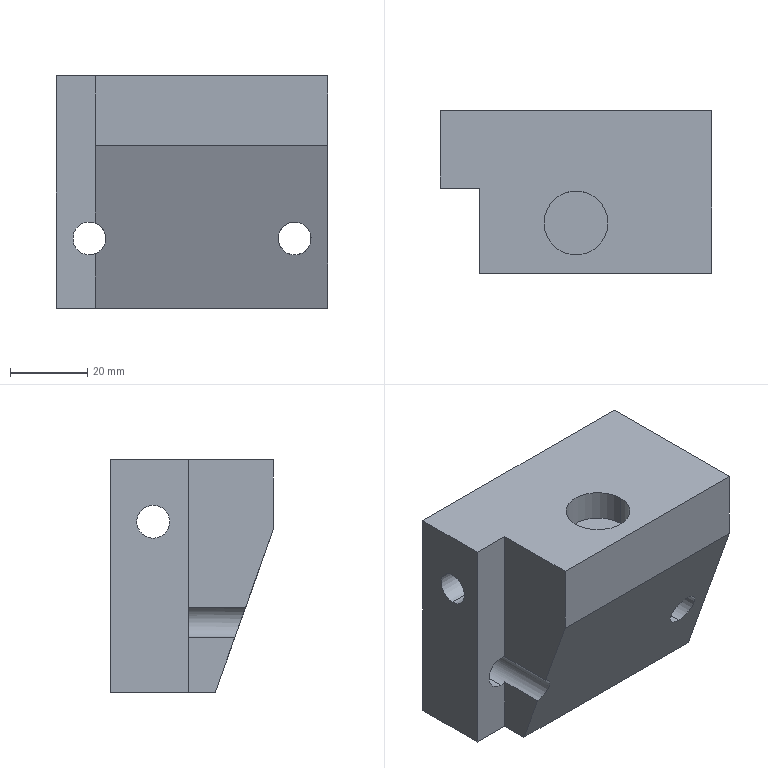Part | SolidWorks | features ICE 4, Extrusion 1 | 1 solid | 19 faces | box 70 x 42 x 60 mm | volume 135372 mm3 | plane 11 | cylinder 8 | commonest cylinder face diameters 8.5 x6 16.5 x2
STEP:
#1=CARTESIAN_POINT('',(-8.25,-9.,22.));
#2=VERTEX_POINT('',#1);
#3=CARTESIAN_POINT('',(8.25,-9.,22.));
#4=VERTEX_POINT('',#3);
#5=CARTESIAN_POINT('',(0.,-9.,22.));
#6=DIRECTION('',(0.,0.,1.));
#7=DIRECTION('',(1.,0.,0.));
#8=AXIS2_PLACEMENT_3D('',#5,#6,#7);
#9=CIRCLE('',#8,8.25);
#10=EDGE_CURVE('',#2,#4,#9,.T.);
#11=ORIENTED_EDGE('',*,*,#10,.F.);
#12=CARTESIAN_POINT('',(-8.25,-9.,30.));
#13=VERTEX_POINT('',#12);
#14=CARTESIAN_POINT('',(-8.25,-9.,22.));
#15=DIRECTION('',(0.,0.,1.));
#16=VECTOR('',#15,1000.);
#17=LINE('',#14,#16);
#18=EDGE_CURVE('',#2,#13,#17,.T.);
#19=ORIENTED_EDGE('',*,*,#18,.T.);
#20=CARTESIAN_POINT('',(8.25,-9.,30.));
#21=VERTEX_POINT('',#20);
#22=CARTESIAN_POINT('',(0.,-9.,30.));
#23=DIRECTION('',(0.,0.,1.));
#24=DIRECTION('',(1.,0.,0.));
#25=AXIS2_PLACEMENT_3D('',#22,#23,#24);
#26=CIRCLE('',#25,8.25);
#27=EDGE_CURVE('',#13,#21,#26,.T.);
#28=ORIENTED_EDGE('',*,*,#27,.T.);
#29=CARTESIAN_POINT('',(8.25,-9.,22.));
#30=DIRECTION('',(0.,0.,1.));
#31=VECTOR('',#30,1000.);
#32=LINE('',#29,#31);
#33=EDGE_CURVE('',#4,#21,#32,.T.);
#34=ORIENTED_EDGE('',*,*,#33,.F.);
#35=EDGE_LOOP('',(#11,#19,#28,#34));
#36=FACE_OUTER_BOUND('',#35,.T.);
#37=CARTESIAN_POINT('',(0.,-9.,22.));
#38=DIRECTION('',(0.,0.,1.));
#39=DIRECTION('',(1.,0.,0.));
#40=AXIS2_PLACEMENT_3D('',#37,#38,#39);
#41=CYLINDRICAL_SURFACE('',#40,8.25);
#42=ADVANCED_FACE('',(#36),#41,.F.);
#43=CARTESIAN_POINT('',(26.5,-14.946,-7.75));
#44=VERTEX_POINT('',#43);
#45=CARTESIAN_POINT('',(26.5,-11.911,-16.25));
#46=VERTEX_POINT('',#45);
#47=CARTESIAN_POINT('',(26.5,-14.946,-7.75));
#48=CARTESIAN_POINT('',(18.,-14.946,-7.75));
#49=CARTESIAN_POINT('',(18.,-11.911,-16.25));
#50=CARTESIAN_POINT('',(26.5,-11.911,-16.25));
#51=(BOUNDED_CURVE()B_SPLINE_CURVE(3,(#47,#48,#49,#50),.UNSPECIFIED.,.F.,.F.)B_SPLINE_CURVE_WITH_KNOTS((4,4),(3.142,6.283),.UNSPECIFIED.)CURVE()GEOMETRIC_REPRESENTATION_ITEM()RATIONAL_B_SPLINE_CURVE((1.,0.3333,0.3333,1.))REPRESENTATION_ITEM(''));
#52=EDGE_CURVE('',#44,#46,#51,.T.);
#53=ORIENTED_EDGE('',*,*,#52,.T.);
#54=CARTESIAN_POINT('',(26.5,20.,-16.25));
#55=VERTEX_POINT('',#54);
#56=CARTESIAN_POINT('',(26.5,-71.,-16.25));
#57=DIRECTION('',(0.,1.,0.));
#58=VECTOR('',#57,1000.);
#59=LINE('',#56,#58);
#60=EDGE_CURVE('',#46,#55,#59,.T.);
#61=ORIENTED_EDGE('',*,*,#60,.T.);
#62=CARTESIAN_POINT('',(26.5,20.,-7.75));
#63=VERTEX_POINT('',#62);
#64=CARTESIAN_POINT('',(26.5,20.,-12.));
#65=DIRECTION('',(0.,1.,0.));
#66=DIRECTION('',(0.,0.,1.));
#67=AXIS2_PLACEMENT_3D('',#64,#65,#66);
#68=CIRCLE('',#67,4.25);
#69=EDGE_CURVE('',#55,#63,#68,.T.);
#70=ORIENTED_EDGE('',*,*,#69,.T.);
#71=CARTESIAN_POINT('',(26.5,-71.,-7.75));
#72=DIRECTION('',(0.,1.,0.));
#73=VECTOR('',#72,1000.);
#74=LINE('',#71,#73);
#75=EDGE_CURVE('',#44,#63,#74,.T.);
#76=ORIENTED_EDGE('',*,*,#75,.F.);
#77=EDGE_LOOP('',(#53,#61,#70,#76));
#78=FACE_OUTER_BOUND('',#77,.T.);
#79=CARTESIAN_POINT('',(26.5,-71.,-12.));
#80=DIRECTION('',(0.,1.,0.));
#81=DIRECTION('',(0.,0.,1.));
#82=AXIS2_PLACEMENT_3D('',#79,#80,#81);
#83=CYLINDRICAL_SURFACE('',#82,4.25);
#84=ADVANCED_FACE('',(#78),#83,.F.);
#85=CARTESIAN_POINT('',(-26.5,0.,-16.25));
#86=VERTEX_POINT('',#85);
#87=CARTESIAN_POINT('',(-26.5,0.,-7.75));
#88=VERTEX_POINT('',#87);
#89=CARTESIAN_POINT('',(-26.5,0.,-12.));
#90=DIRECTION('',(0.,1.,0.));
#91=DIRECTION('',(0.,0.,1.));
#92=AXIS2_PLACEMENT_3D('',#89,#90,#91);
#93=CIRCLE('',#92,4.25);
#94=EDGE_CURVE('',#86,#88,#93,.T.);
#95=ORIENTED_EDGE('',*,*,#94,.F.);
#96=CARTESIAN_POINT('',(-26.5,20.,-16.25));
#97=VERTEX_POINT('',#96);
#98=CARTESIAN_POINT('',(-26.5,-71.,-16.25));
#99=DIRECTION('',(0.,1.,0.));
#100=VECTOR('',#99,1000.);
#101=LINE('',#98,#100);
#102=EDGE_CURVE('',#86,#97,#101,.T.);
#103=ORIENTED_EDGE('',*,*,#102,.T.);
#104=CARTESIAN_POINT('',(-26.5,20.,-7.75));
#105=VERTEX_POINT('',#104);
#106=CARTESIAN_POINT('',(-26.5,20.,-12.));
#107=DIRECTION('',(0.,1.,0.));
#108=DIRECTION('',(0.,0.,-1.));
#109=AXIS2_PLACEMENT_3D('',#106,#107,#108);
#110=CIRCLE('',#109,4.25);
#111=EDGE_CURVE('',#97,#105,#110,.T.);
#112=ORIENTED_EDGE('',*,*,#111,.T.);
#113=CARTESIAN_POINT('',(-26.5,-71.,-7.75));
#114=DIRECTION('',(0.,1.,0.));
#115=VECTOR('',#114,1000.);
#116=LINE('',#113,#115);
#117=EDGE_CURVE('',#88,#105,#116,.T.);
#118=ORIENTED_EDGE('',*,*,#117,.F.);
#119=EDGE_LOOP('',(#95,#103,#112,#118));
#120=FACE_OUTER_BOUND('',#119,.T.);
#121=CARTESIAN_POINT('',(-26.5,-71.,-12.));
#122=DIRECTION('',(0.,1.,0.));
#123=DIRECTION('',(0.,0.,1.));
#124=AXIS2_PLACEMENT_3D('',#121,#122,#123);
#125=CYLINDRICAL_SURFACE('',#124,4.25);
#126=ADVANCED_FACE('',(#120),#125,.F.);
#127=CARTESIAN_POINT('',(35.,9.,9.75));
#128=VERTEX_POINT('',#127);
#129=CARTESIAN_POINT('',(35.,9.,18.25));
#130=VERTEX_POINT('',#129);
#131=CARTESIAN_POINT('',(35.,9.,14.));
#132=DIRECTION('',(-1.,0.,0.));
#133=DIRECTION('',(0.,0.,1.));
#134=AXIS2_PLACEMENT_3D('',#131,#132,#133);
#135=CIRCLE('',#134,4.25);
#136=EDGE_CURVE('',#128,#130,#135,.T.);
#137=ORIENTED_EDGE('',*,*,#136,.F.);
#138=CARTESIAN_POINT('',(-35.,9.,9.75));
#139=VERTEX_POINT('',#138);
#140=CARTESIAN_POINT('',(96.,9.,9.75));
#141=DIRECTION('',(-1.,0.,0.));
#142=VECTOR('',#141,1000.);
#143=LINE('',#140,#142);
#144=EDGE_CURVE('',#128,#139,#143,.T.);
#145=ORIENTED_EDGE('',*,*,#144,.T.);
#146=CARTESIAN_POINT('',(-35.,9.,18.25));
#147=VERTEX_POINT('',#146);
#148=CARTESIAN_POINT('',(-35.,9.,14.));
#149=DIRECTION('',(-1.,0.,0.));
#150=DIRECTION('',(0.,0.,1.));
#151=AXIS2_PLACEMENT_3D('',#148,#149,#150);
#152=CIRCLE('',#151,4.25);
#153=EDGE_CURVE('',#139,#147,#152,.T.);
#154=ORIENTED_EDGE('',*,*,#153,.T.);
#155=CARTESIAN_POINT('',(96.,9.,18.25));
#156=DIRECTION('',(-1.,0.,0.));
#157=VECTOR('',#156,1000.);
#158=LINE('',#155,#157);
#159=EDGE_CURVE('',#130,#147,#158,.T.);
#160=ORIENTED_EDGE('',*,*,#159,.F.);
#161=EDGE_LOOP('',(#137,#145,#154,#160));
#162=FACE_OUTER_BOUND('',#161,.T.);
#163=CARTESIAN_POINT('',(96.,9.,14.));
#164=DIRECTION('',(-1.,0.,0.));
#165=DIRECTION('',(0.,0.,1.));
#166=AXIS2_PLACEMENT_3D('',#163,#164,#165);
#167=CYLINDRICAL_SURFACE('',#166,4.25);
#168=ADVANCED_FACE('',(#162),#167,.F.);
#169=CARTESIAN_POINT('',(-25.,-14.849,-8.024));
#170=VERTEX_POINT('',#169);
#171=CARTESIAN_POINT('',(-25.,0.,-8.024));
#172=VERTEX_POINT('',#171);
#173=CARTESIAN_POINT('',(-25.,-71.,-8.024));
#174=DIRECTION('',(0.,1.,0.));
#175=VECTOR('',#174,1000.);
#176=LINE('',#173,#175);
#177=EDGE_CURVE('',#170,#172,#176,.T.);
#178=ORIENTED_EDGE('',*,*,#177,.F.);
#179=CARTESIAN_POINT('',(-25.,-22.,12.));
#180=VERTEX_POINT('',#179);
#181=CARTESIAN_POINT('',(-25.,-7.,-30.));
#182=DIRECTION('',(0.,0.3363,-0.9417));
#183=VECTOR('',#182,1000.);
#184=LINE('',#181,#183);
#185=EDGE_CURVE('',#180,#170,#184,.T.);
#186=ORIENTED_EDGE('',*,*,#185,.F.);
#187=CARTESIAN_POINT('',(-25.,-22.,30.));
#188=VERTEX_POINT('',#187);
#189=CARTESIAN_POINT('',(-25.,-22.,12.));
#190=DIRECTION('',(0.,0.,-1.));
#191=VECTOR('',#190,1000.);
#192=LINE('',#189,#191);
#193=EDGE_CURVE('',#188,#180,#192,.T.);
#194=ORIENTED_EDGE('',*,*,#193,.F.);
#195=CARTESIAN_POINT('',(-25.,0.,30.));
#196=VERTEX_POINT('',#195);
#197=CARTESIAN_POINT('',(-25.,-22.,30.));
#198=DIRECTION('',(0.,-1.,0.));
#199=VECTOR('',#198,1000.);
#200=LINE('',#197,#199);
#201=EDGE_CURVE('',#196,#188,#200,.T.);
#202=ORIENTED_EDGE('',*,*,#201,.F.);
#203=CARTESIAN_POINT('',(-25.,0.,0.));
#204=DIRECTION('',(0.,0.,1.));
#205=VECTOR('',#204,1000.);
#206=LINE('',#203,#205);
#207=EDGE_CURVE('',#172,#196,#206,.T.);
#208=ORIENTED_EDGE('',*,*,#207,.F.);
#209=EDGE_LOOP('',(#178,#186,#194,#202,#208));
#210=FACE_OUTER_BOUND('',#209,.T.);
#211=CARTESIAN_POINT('',(-25.,0.,0.));
#212=DIRECTION('',(-1.,0.,0.));
#213=DIRECTION('',(0.,0.,1.));
#214=AXIS2_PLACEMENT_3D('',#211,#212,#213);
#215=PLANE('',#214);
#216=ADVANCED_FACE('',(#210),#215,.T.);
#217=CARTESIAN_POINT('',(35.,9.,14.));
#218=DIRECTION('',(-1.,0.,0.));
#219=DIRECTION('',(0.,0.,1.));
#220=AXIS2_PLACEMENT_3D('',#217,#218,#219);
#221=CIRCLE('',#220,4.25);
#222=EDGE_CURVE('',#130,#128,#221,.T.);
#223=ORIENTED_EDGE('',*,*,#222,.T.);
#224=ORIENTED_EDGE('',*,*,#136,.T.);
#225=EDGE_LOOP('',(#223,#224));
#226=FACE_BOUND('',#225,.T.);
#227=CARTESIAN_POINT('',(35.,20.,30.));
#228=VERTEX_POINT('',#227);
#229=CARTESIAN_POINT('',(35.,-22.,30.));
#230=VERTEX_POINT('',#229);
#231=CARTESIAN_POINT('',(35.,20.,30.));
#232=DIRECTION('',(0.,-1.,0.));
#233=VECTOR('',#232,1000.);
#234=LINE('',#231,#233);
#235=EDGE_CURVE('',#228,#230,#234,.T.);
#236=ORIENTED_EDGE('',*,*,#235,.T.);
#237=CARTESIAN_POINT('',(35.,-22.,12.));
#238=VERTEX_POINT('',#237);
#239=CARTESIAN_POINT('',(35.,-22.,12.));
#240=DIRECTION('',(0.,0.,-1.));
#241=VECTOR('',#240,1000.);
#242=LINE('',#239,#241);
#243=EDGE_CURVE('',#230,#238,#242,.T.);
#244=ORIENTED_EDGE('',*,*,#243,.T.);
#245=CARTESIAN_POINT('',(35.,-7.,-30.));
#246=VERTEX_POINT('',#245);
#247=CARTESIAN_POINT('',(35.,-7.,-30.));
#248=DIRECTION('',(0.,0.3363,-0.9417));
#249=VECTOR('',#248,1000.);
#250=LINE('',#247,#249);
#251=EDGE_CURVE('',#238,#246,#250,.T.);
#252=ORIENTED_EDGE('',*,*,#251,.T.);
#253=CARTESIAN_POINT('',(35.,20.,-30.));
#254=VERTEX_POINT('',#253);
#255=CARTESIAN_POINT('',(35.,20.,-30.));
#256=DIRECTION('',(0.,-1.,0.));
#257=VECTOR('',#256,1000.);
#258=LINE('',#255,#257);
#259=EDGE_CURVE('',#254,#246,#258,.T.);
#260=ORIENTED_EDGE('',*,*,#259,.F.);
#261=CARTESIAN_POINT('',(35.,20.,-30.));
#262=DIRECTION('',(0.,0.,-1.));
#263=VECTOR('',#262,1000.);
#264=LINE('',#261,#263);
#265=EDGE_CURVE('',#228,#254,#264,.T.);
#266=ORIENTED_EDGE('',*,*,#265,.F.);
#267=EDGE_LOOP('',(#236,#244,#252,#260,#266));
#268=FACE_OUTER_BOUND('',#267,.T.);
#269=CARTESIAN_POINT('',(35.,20.,-30.));
#270=DIRECTION('',(-1.,0.,0.));
#271=DIRECTION('',(0.,0.,1.));
#272=AXIS2_PLACEMENT_3D('',#269,#270,#271);
#273=PLANE('',#272);
#274=ADVANCED_FACE('',(#226,#268),#273,.F.);
#275=CARTESIAN_POINT('',(-35.,20.,-30.));
#276=VERTEX_POINT('',#275);
#277=CARTESIAN_POINT('',(-35.,0.,-30.));
#278=VERTEX_POINT('',#277);
#279=CARTESIAN_POINT('',(-35.,20.,-30.));
#280=DIRECTION('',(0.,-1.,0.));
#281=VECTOR('',#280,1000.);
#282=LINE('',#279,#281);
#283=EDGE_CURVE('',#276,#278,#282,.T.);
#284=ORIENTED_EDGE('',*,*,#283,.F.);
#285=CARTESIAN_POINT('',(-35.,20.,-30.));
#286=DIRECTION('',(-1.,0.,0.));
#287=VECTOR('',#286,1000.);
#288=LINE('',#285,#287);
#289=EDGE_CURVE('',#254,#276,#288,.T.);
#290=ORIENTED_EDGE('',*,*,#289,.F.);
#291=ORIENTED_EDGE('',*,*,#259,.T.);
#292=CARTESIAN_POINT('',(-25.,-7.,-30.));
#293=VERTEX_POINT('',#292);
#294=CARTESIAN_POINT('',(-25.,-7.,-30.));
#295=DIRECTION('',(1.,0.,0.));
#296=VECTOR('',#295,1000.);
#297=LINE('',#294,#296);
#298=EDGE_CURVE('',#293,#246,#297,.T.);
#299=ORIENTED_EDGE('',*,*,#298,.F.);
#300=CARTESIAN_POINT('',(-25.,0.,-30.));
#301=VERTEX_POINT('',#300);
#302=CARTESIAN_POINT('',(-25.,0.,-30.));
#303=DIRECTION('',(0.,1.,0.));
#304=VECTOR('',#303,1000.);
#305=LINE('',#302,#304);
#306=EDGE_CURVE('',#293,#301,#305,.T.);
#307=ORIENTED_EDGE('',*,*,#306,.T.);
#308=CARTESIAN_POINT('',(-35.,0.,-30.));
#309=DIRECTION('',(-1.,0.,0.));
#310=VECTOR('',#309,1000.);
#311=LINE('',#308,#310);
#312=EDGE_CURVE('',#301,#278,#311,.T.);
#313=ORIENTED_EDGE('',*,*,#312,.T.);
#314=EDGE_LOOP('',(#284,#290,#291,#299,#307,#313));
#315=FACE_OUTER_BOUND('',#314,.T.);
#316=CARTESIAN_POINT('',(-35.,20.,-30.));
#317=DIRECTION('',(0.,0.,1.));
#318=DIRECTION('',(1.,0.,0.));
#319=AXIS2_PLACEMENT_3D('',#316,#317,#318);
#320=PLANE('',#319);
#321=ADVANCED_FACE('',(#315),#320,.F.);
#322=CARTESIAN_POINT('',(-35.,9.,14.));
#323=DIRECTION('',(-1.,0.,0.));
#324=DIRECTION('',(0.,0.,1.));
#325=AXIS2_PLACEMENT_3D('',#322,#323,#324);
#326=CIRCLE('',#325,4.25);
#327=EDGE_CURVE('',#147,#139,#326,.T.);
#328=ORIENTED_EDGE('',*,*,#327,.F.);
#329=ORIENTED_EDGE('',*,*,#153,.F.);
#330=EDGE_LOOP('',(#328,#329));
#331=FACE_BOUND('',#330,.T.);
#332=CARTESIAN_POINT('',(-35.,0.,30.));
#333=VERTEX_POINT('',#332);
#334=CARTESIAN_POINT('',(-35.,0.,-30.));
#335=DIRECTION('',(0.,0.,1.));
#336=VECTOR('',#335,1000.);
#337=LINE('',#334,#336);
#338=EDGE_CURVE('',#278,#333,#337,.T.);
#339=ORIENTED_EDGE('',*,*,#338,.T.);
#340=CARTESIAN_POINT('',(-35.,20.,30.));
#341=VERTEX_POINT('',#340);
#342=CARTESIAN_POINT('',(-35.,20.,30.));
#343=DIRECTION('',(0.,-1.,0.));
#344=VECTOR('',#343,1000.);
#345=LINE('',#342,#344);
#346=EDGE_CURVE('',#341,#333,#345,.T.);
#347=ORIENTED_EDGE('',*,*,#346,.F.);
#348=CARTESIAN_POINT('',(-35.,20.,-30.));
#349=DIRECTION('',(0.,0.,1.));
#350=VECTOR('',#349,1000.);
#351=LINE('',#348,#350);
#352=EDGE_CURVE('',#276,#341,#351,.T.);
#353=ORIENTED_EDGE('',*,*,#352,.F.);
#354=ORIENTED_EDGE('',*,*,#283,.T.);
#355=EDGE_LOOP('',(#339,#347,#353,#354));
#356=FACE_OUTER_BOUND('',#355,.T.);
#357=CARTESIAN_POINT('',(-35.,20.,-30.));
#358=DIRECTION('',(1.,0.,0.));
#359=DIRECTION('',(0.,0.,-1.));
#360=AXIS2_PLACEMENT_3D('',#357,#358,#359);
#361=PLANE('',#360);
#362=ADVANCED_FACE('',(#331,#356),#361,.F.);
#363=CARTESIAN_POINT('',(0.,-9.,30.));
#364=DIRECTION('',(0.,0.,1.));
#365=DIRECTION('',(1.,0.,0.));
#366=AXIS2_PLACEMENT_3D('',#363,#364,#365);
#367=CIRCLE('',#366,8.25);
#368=EDGE_CURVE('',#21,#13,#367,.T.);
#369=ORIENTED_EDGE('',*,*,#368,.F.);
#370=ORIENTED_EDGE('',*,*,#27,.F.);
#371=EDGE_LOOP('',(#369,#370));
#372=FACE_BOUND('',#371,.T.);
#373=CARTESIAN_POINT('',(-35.,0.,30.));
#374=DIRECTION('',(1.,0.,0.));
#375=VECTOR('',#374,1000.);
#376=LINE('',#373,#375);
#377=EDGE_CURVE('',#333,#196,#376,.T.);
#378=ORIENTED_EDGE('',*,*,#377,.T.);
#379=ORIENTED_EDGE('',*,*,#201,.T.);
#380=CARTESIAN_POINT('',(-25.,-22.,30.));
#381=DIRECTION('',(1.,0.,0.));
#382=VECTOR('',#381,1000.);
#383=LINE('',#380,#382);
#384=EDGE_CURVE('',#188,#230,#383,.T.);
#385=ORIENTED_EDGE('',*,*,#384,.T.);
#386=ORIENTED_EDGE('',*,*,#235,.F.);
#387=CARTESIAN_POINT('',(-35.,20.,30.));
#388=DIRECTION('',(1.,0.,0.));
#389=VECTOR('',#388,1000.);
#390=LINE('',#387,#389);
#391=EDGE_CURVE('',#341,#228,#390,.T.);
#392=ORIENTED_EDGE('',*,*,#391,.F.);
#393=ORIENTED_EDGE('',*,*,#346,.T.);
#394=EDGE_LOOP('',(#378,#379,#385,#386,#392,#393));
#395=FACE_OUTER_BOUND('',#394,.T.);
#396=CARTESIAN_POINT('',(-35.,20.,30.));
#397=DIRECTION('',(0.,0.,-1.));
#398=DIRECTION('',(-1.,0.,0.));
#399=AXIS2_PLACEMENT_3D('',#396,#397,#398);
#400=PLANE('',#399);
#401=ADVANCED_FACE('',(#372,#395),#400,.F.);
#402=CARTESIAN_POINT('',(26.5,20.,-12.));
#403=DIRECTION('',(0.,1.,0.));
#404=DIRECTION('',(0.,0.,1.));
#405=AXIS2_PLACEMENT_3D('',#402,#403,#404);
#406=CIRCLE('',#405,4.25);
#407=EDGE_CURVE('',#63,#55,#406,.T.);
#408=ORIENTED_EDGE('',*,*,#407,.F.);
#409=ORIENTED_EDGE('',*,*,#69,.F.);
#410=EDGE_LOOP('',(#408,#409));
#411=FACE_BOUND('',#410,.T.);
#412=CARTESIAN_POINT('',(-26.5,20.,-12.));
#413=DIRECTION('',(0.,1.,0.));
#414=DIRECTION('',(0.,0.,-1.));
#415=AXIS2_PLACEMENT_3D('',#412,#413,#414);
#416=CIRCLE('',#415,4.25);
#417=EDGE_CURVE('',#105,#97,#416,.T.);
#418=ORIENTED_EDGE('',*,*,#417,.F.);
#419=ORIENTED_EDGE('',*,*,#111,.F.);
#420=EDGE_LOOP('',(#418,#419));
#421=FACE_BOUND('',#420,.T.);
#422=ORIENTED_EDGE('',*,*,#391,.T.);
#423=ORIENTED_EDGE('',*,*,#265,.T.);
#424=ORIENTED_EDGE('',*,*,#289,.T.);
#425=ORIENTED_EDGE('',*,*,#352,.T.);
#426=EDGE_LOOP('',(#422,#423,#424,#425));
#427=FACE_OUTER_BOUND('',#426,.T.);
#428=CARTESIAN_POINT('',(0.,20.,0.));
#429=DIRECTION('',(0.,1.,0.));
#430=DIRECTION('',(0.,0.,1.));
#431=AXIS2_PLACEMENT_3D('',#428,#429,#430);
#432=PLANE('',#431);
#433=ADVANCED_FACE('',(#411,#421,#427),#432,.T.);
#434=CARTESIAN_POINT('',(-25.,0.,-15.976));
#435=VERTEX_POINT('',#434);
#436=CARTESIAN_POINT('',(-25.,0.,0.));
#437=DIRECTION('',(0.,0.,1.));
#438=VECTOR('',#437,1000.);
#439=LINE('',#436,#438);
#440=EDGE_CURVE('',#301,#435,#439,.T.);
#441=ORIENTED_EDGE('',*,*,#440,.T.);
#442=CARTESIAN_POINT('',(-26.5,0.,-12.));
#443=DIRECTION('',(0.,1.,0.));
#444=DIRECTION('',(0.,0.,1.));
#445=AXIS2_PLACEMENT_3D('',#442,#443,#444);
#446=CIRCLE('',#445,4.25);
#447=EDGE_CURVE('',#435,#86,#446,.T.);
#448=ORIENTED_EDGE('',*,*,#447,.T.);
#449=ORIENTED_EDGE('',*,*,#94,.T.);
#450=CARTESIAN_POINT('',(-26.5,0.,-12.));
#451=DIRECTION('',(0.,1.,0.));
#452=DIRECTION('',(0.,0.,1.));
#453=AXIS2_PLACEMENT_3D('',#450,#451,#452);
#454=CIRCLE('',#453,4.25);
#455=EDGE_CURVE('',#88,#172,#454,.T.);
#456=ORIENTED_EDGE('',*,*,#455,.T.);
#457=ORIENTED_EDGE('',*,*,#207,.T.);
#458=ORIENTED_EDGE('',*,*,#377,.F.);
#459=ORIENTED_EDGE('',*,*,#338,.F.);
#460=ORIENTED_EDGE('',*,*,#312,.F.);
#461=EDGE_LOOP('',(#441,#448,#449,#456,#457,#458,#459,#460));
#462=FACE_OUTER_BOUND('',#461,.T.);
#463=CARTESIAN_POINT('',(0.,0.,0.));
#464=DIRECTION('',(0.,1.,0.));
#465=DIRECTION('',(0.,0.,1.));
#466=AXIS2_PLACEMENT_3D('',#463,#464,#465);
#467=PLANE('',#466);
#468=ADVANCED_FACE('',(#462),#467,.F.);
#469=CARTESIAN_POINT('',(-25.,-12.008,-15.976));
#470=VERTEX_POINT('',#469);
#471=CARTESIAN_POINT('',(-25.,-71.,-15.976));
#472=DIRECTION('',(0.,-1.,0.));
#473=VECTOR('',#472,1000.);
#474=LINE('',#471,#473);
#475=EDGE_CURVE('',#435,#470,#474,.T.);
#476=ORIENTED_EDGE('',*,*,#475,.F.);
#477=ORIENTED_EDGE('',*,*,#440,.F.);
#478=ORIENTED_EDGE('',*,*,#306,.F.);
#479=CARTESIAN_POINT('',(-25.,-7.,-30.));
#480=DIRECTION('',(0.,0.3363,-0.9417));
#481=VECTOR('',#480,1000.);
#482=LINE('',#479,#481);
#483=EDGE_CURVE('',#470,#293,#482,.T.);
#484=ORIENTED_EDGE('',*,*,#483,.F.);
#485=EDGE_LOOP('',(#476,#477,#478,#484));
#486=FACE_OUTER_BOUND('',#485,.T.);
#487=CARTESIAN_POINT('',(-25.,0.,0.));
#488=DIRECTION('',(-1.,0.,0.));
#489=DIRECTION('',(0.,0.,1.));
#490=AXIS2_PLACEMENT_3D('',#487,#488,#489);
#491=PLANE('',#490);
#492=ADVANCED_FACE('',(#486),#491,.T.);
#493=ORIENTED_EDGE('',*,*,#52,.F.);
#494=CARTESIAN_POINT('',(26.5,-11.911,-16.25));
#495=CARTESIAN_POINT('',(35.,-11.911,-16.25));
#496=CARTESIAN_POINT('',(35.,-14.946,-7.75));
#497=CARTESIAN_POINT('',(26.5,-14.946,-7.75));
#498=(BOUNDED_CURVE()B_SPLINE_CURVE(3,(#494,#495,#496,#497),.UNSPECIFIED.,.F.,.F.)B_SPLINE_CURVE_WITH_KNOTS((4,4),(0.,3.142),.UNSPECIFIED.)CURVE()GEOMETRIC_REPRESENTATION_ITEM()RATIONAL_B_SPLINE_CURVE((1.,0.3333,0.3333,1.))REPRESENTATION_ITEM(''));
#499=EDGE_CURVE('',#46,#44,#498,.T.);
#500=ORIENTED_EDGE('',*,*,#499,.F.);
#501=EDGE_LOOP('',(#493,#500));
#502=FACE_BOUND('',#501,.T.);
#503=CARTESIAN_POINT('',(-25.,-12.008,-15.976));
#504=CARTESIAN_POINT('',(-20.638,-12.596,-14.331));
#505=CARTESIAN_POINT('',(-20.638,-14.261,-9.669));
#506=CARTESIAN_POINT('',(-25.,-14.849,-8.024));
#507=(BOUNDED_CURVE()B_SPLINE_CURVE(3,(#503,#504,#505,#506),.UNSPECIFIED.,.F.,.F.)B_SPLINE_CURVE_WITH_KNOTS((4,4),(0.3607,2.781),.UNSPECIFIED.)CURVE()GEOMETRIC_REPRESENTATION_ITEM()RATIONAL_B_SPLINE_CURVE((1.,0.5686,0.5686,1.))REPRESENTATION_ITEM(''));
#508=EDGE_CURVE('',#470,#170,#507,.T.);
#509=ORIENTED_EDGE('',*,*,#508,.F.);
#510=ORIENTED_EDGE('',*,*,#483,.T.);
#511=ORIENTED_EDGE('',*,*,#298,.T.);
#512=ORIENTED_EDGE('',*,*,#251,.F.);
#513=CARTESIAN_POINT('',(-25.,-22.,12.));
#514=DIRECTION('',(1.,0.,0.));
#515=VECTOR('',#514,1000.);
#516=LINE('',#513,#515);
#517=EDGE_CURVE('',#180,#238,#516,.T.);
#518=ORIENTED_EDGE('',*,*,#517,.F.);
#519=ORIENTED_EDGE('',*,*,#185,.T.);
#520=EDGE_LOOP('',(#509,#510,#511,#512,#518,#519));
#521=FACE_OUTER_BOUND('',#520,.T.);
#522=CARTESIAN_POINT('',(-25.,-7.,-30.));
#523=DIRECTION('',(0.,-0.9417,-0.3363));
#524=DIRECTION('',(0.,0.3363,-0.9417));
#525=AXIS2_PLACEMENT_3D('',#522,#523,#524);
#526=PLANE('',#525);
#527=ADVANCED_FACE('',(#502,#521),#526,.T.);
#528=ORIENTED_EDGE('',*,*,#243,.F.);
#529=ORIENTED_EDGE('',*,*,#384,.F.);
#530=ORIENTED_EDGE('',*,*,#193,.T.);
#531=ORIENTED_EDGE('',*,*,#517,.T.);
#532=EDGE_LOOP('',(#528,#529,#530,#531));
#533=FACE_OUTER_BOUND('',#532,.T.);
#534=CARTESIAN_POINT('',(-25.,-22.,12.));
#535=DIRECTION('',(0.,-1.,0.));
#536=DIRECTION('',(0.,0.,-1.));
#537=AXIS2_PLACEMENT_3D('',#534,#535,#536);
#538=PLANE('',#537);
#539=ADVANCED_FACE('',(#533),#538,.T.);
#540=ORIENTED_EDGE('',*,*,#144,.F.);
#541=ORIENTED_EDGE('',*,*,#222,.F.);
#542=ORIENTED_EDGE('',*,*,#159,.T.);
#543=ORIENTED_EDGE('',*,*,#327,.T.);
#544=EDGE_LOOP('',(#540,#541,#542,#543));
#545=FACE_OUTER_BOUND('',#544,.T.);
#546=CARTESIAN_POINT('',(96.,9.,14.));
#547=DIRECTION('',(-1.,0.,0.));
#548=DIRECTION('',(0.,0.,1.));
#549=AXIS2_PLACEMENT_3D('',#546,#547,#548);
#550=CYLINDRICAL_SURFACE('',#549,4.25);
#551=ADVANCED_FACE('',(#545),#550,.F.);
#552=ORIENTED_EDGE('',*,*,#102,.F.);
#553=ORIENTED_EDGE('',*,*,#447,.F.);
#554=ORIENTED_EDGE('',*,*,#475,.T.);
#555=ORIENTED_EDGE('',*,*,#508,.T.);
#556=ORIENTED_EDGE('',*,*,#177,.T.);
#557=ORIENTED_EDGE('',*,*,#455,.F.);
#558=ORIENTED_EDGE('',*,*,#117,.T.);
#559=ORIENTED_EDGE('',*,*,#417,.T.);
#560=EDGE_LOOP('',(#552,#553,#554,#555,#556,#557,#558,#559));
#561=FACE_OUTER_BOUND('',#560,.T.);
#562=CARTESIAN_POINT('',(-26.5,-71.,-12.));
#563=DIRECTION('',(0.,1.,0.));
#564=DIRECTION('',(0.,0.,1.));
#565=AXIS2_PLACEMENT_3D('',#562,#563,#564);
#566=CYLINDRICAL_SURFACE('',#565,4.25);
#567=ADVANCED_FACE('',(#561),#566,.F.);
#568=ORIENTED_EDGE('',*,*,#60,.F.);
#569=ORIENTED_EDGE('',*,*,#499,.T.);
#570=ORIENTED_EDGE('',*,*,#75,.T.);
#571=ORIENTED_EDGE('',*,*,#407,.T.);
#572=EDGE_LOOP('',(#568,#569,#570,#571));
#573=FACE_OUTER_BOUND('',#572,.T.);
#574=CARTESIAN_POINT('',(26.5,-71.,-12.));
#575=DIRECTION('',(0.,1.,0.));
#576=DIRECTION('',(0.,0.,1.));
#577=AXIS2_PLACEMENT_3D('',#574,#575,#576);
#578=CYLINDRICAL_SURFACE('',#577,4.25);
#579=ADVANCED_FACE('',(#573),#578,.F.);
#580=ORIENTED_EDGE('',*,*,#18,.F.);
#581=CARTESIAN_POINT('',(0.,-9.,22.));
#582=DIRECTION('',(0.,0.,1.));
#583=DIRECTION('',(1.,0.,0.));
#584=AXIS2_PLACEMENT_3D('',#581,#582,#583);
#585=CIRCLE('',#584,8.25);
#586=EDGE_CURVE('',#4,#2,#585,.T.);
#587=ORIENTED_EDGE('',*,*,#586,.F.);
#588=ORIENTED_EDGE('',*,*,#33,.T.);
#589=ORIENTED_EDGE('',*,*,#368,.T.);
#590=EDGE_LOOP('',(#580,#587,#588,#589));
#591=FACE_OUTER_BOUND('',#590,.T.);
#592=CARTESIAN_POINT('',(0.,-9.,22.));
#593=DIRECTION('',(0.,0.,1.));
#594=DIRECTION('',(1.,0.,0.));
#595=AXIS2_PLACEMENT_3D('',#592,#593,#594);
#596=CYLINDRICAL_SURFACE('',#595,8.25);
#597=ADVANCED_FACE('',(#591),#596,.F.);
#598=ORIENTED_EDGE('',*,*,#586,.T.);
#599=ORIENTED_EDGE('',*,*,#10,.T.);
#600=EDGE_LOOP('',(#598,#599));
#601=FACE_OUTER_BOUND('',#600,.T.);
#602=CARTESIAN_POINT('',(0.,-9.,22.));
#603=DIRECTION('',(0.,0.,1.));
#604=DIRECTION('',(1.,0.,0.));
#605=AXIS2_PLACEMENT_3D('',#602,#603,#604);
#606=PLANE('',#605);
#607=ADVANCED_FACE('',(#601),#606,.T.);
#608=CLOSED_SHELL('',(#42,#84,#126,#168,#216,#274,#321,#362,#401,#433,#468,#492,#527,#539,#551,#567,#579,#597,#607));
#609=MANIFOLD_SOLID_BREP('',#608);
#610=CARTESIAN_POINT('',(0.,0.,0.));
#611=DIRECTION('',(0.,0.,1.));
#612=DIRECTION('',(1.,0.,0.));
#613=AXIS2_PLACEMENT_3D('',#610,#611,#612);
#614=(LENGTH_UNIT()NAMED_UNIT(*)SI_UNIT(.MILLI.,.METRE.));
#615=UNCERTAINTY_MEASURE_WITH_UNIT(LENGTH_MEASURE(0.00001),#614,'','');
#616=(NAMED_UNIT(*)PLANE_ANGLE_UNIT()SI_UNIT($,.RADIAN.));
#617=(NAMED_UNIT(*)SI_UNIT($,.STERADIAN.)SOLID_ANGLE_UNIT());
#618=(GEOMETRIC_REPRESENTATION_CONTEXT(3)GLOBAL_UNCERTAINTY_ASSIGNED_CONTEXT((#615))GLOBAL_UNIT_ASSIGNED_CONTEXT((#614,#616,#617))REPRESENTATION_CONTEXT('',''));
#619=ADVANCED_BREP_SHAPE_REPRESENTATION('',(#609,#613),#618);